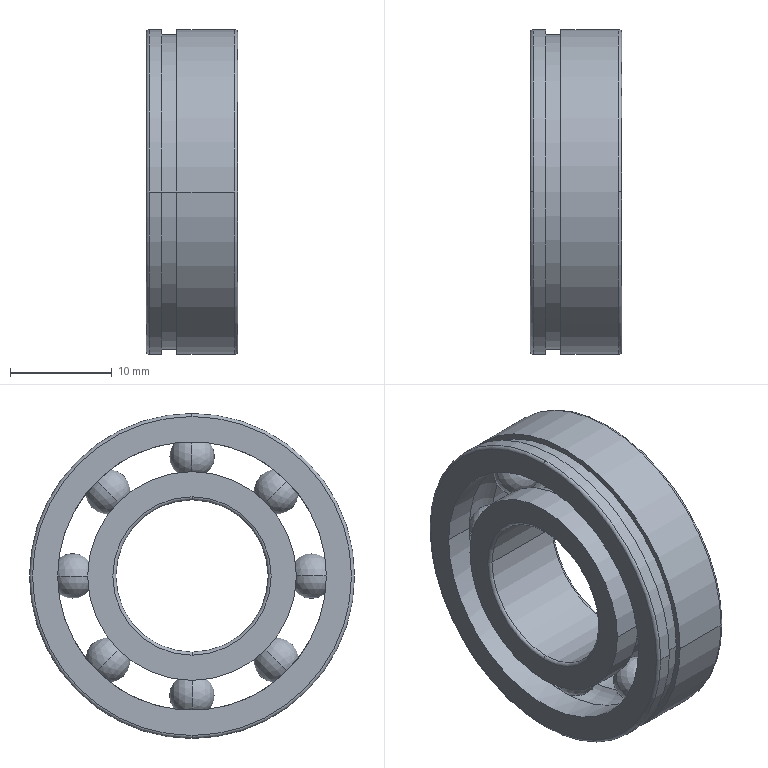Part | SolidWorks | features BaseBody 10 | 10 solids | 52 faces | box 9 x 32 x 32 mm | volume 3713 mm3 | sphere 16 | cylinder 16 | torus 14 | plane 6 | commonest cylinder face diameters 20.542 x4 26.458 x4 32 x4 15 x2 30.92 x2
STEP:
#1=CARTESIAN_POINT('',(4.5,9.54,0.));
#2=VERTEX_POINT('',#1);
#3=CARTESIAN_POINT('',(4.5,13.96,0.));
#4=VERTEX_POINT('',#3);
#5=CARTESIAN_POINT('',(4.5,11.75,0.));
#6=DIRECTION('',(0.,0.,1.));
#7=DIRECTION('',(1.,0.,0.));
#8=AXIS2_PLACEMENT_3D('',#5,#6,#7);
#9=CIRCLE('',#8,2.21);
#10=EDGE_CURVE('',#2,#4,#9,.T.);
#11=ORIENTED_EDGE('',*,*,#10,.F.);
#12=CARTESIAN_POINT('',(4.5,11.75,0.));
#13=DIRECTION('',(0.,0.,-1.));
#14=DIRECTION('',(-1.,0.,0.));
#15=AXIS2_PLACEMENT_3D('',#12,#13,#14);
#16=CIRCLE('',#15,2.21);
#17=EDGE_CURVE('',#2,#4,#16,.T.);
#18=ORIENTED_EDGE('',*,*,#17,.T.);
#19=EDGE_LOOP('',(#11,#18));
#20=FACE_OUTER_BOUND('',#19,.T.);
#21=CARTESIAN_POINT('',(4.5,11.75,0.));
#22=DIRECTION('',(0.,0.,-1.));
#23=DIRECTION('',(1.,0.,0.));
#24=AXIS2_PLACEMENT_3D('',#21,#22,#23);
#25=SPHERICAL_SURFACE('',#24,2.21);
#26=ADVANCED_FACE('',(#20),#25,.T.);
#27=ORIENTED_EDGE('',*,*,#17,.F.);
#28=ORIENTED_EDGE('',*,*,#10,.T.);
#29=EDGE_LOOP('',(#27,#28));
#30=FACE_OUTER_BOUND('',#29,.T.);
#31=CARTESIAN_POINT('',(4.5,11.75,0.));
#32=DIRECTION('',(0.,0.,-1.));
#33=DIRECTION('',(1.,0.,0.));
#34=AXIS2_PLACEMENT_3D('',#31,#32,#33);
#35=SPHERICAL_SURFACE('',#34,2.21);
#36=ADVANCED_FACE('',(#30),#35,.T.);
#37=CLOSED_SHELL('',(#26,#36));
#38=MANIFOLD_SOLID_BREP('',#37);
#39=CARTESIAN_POINT('',(3.,-15.46,0.));
#40=VERTEX_POINT('',#39);
#41=CARTESIAN_POINT('',(3.,15.46,0.));
#42=VERTEX_POINT('',#41);
#43=CARTESIAN_POINT('',(3.,0.,0.));
#44=DIRECTION('',(1.,0.,0.));
#45=DIRECTION('',(0.,1.,0.));
#46=AXIS2_PLACEMENT_3D('',#43,#44,#45);
#47=CIRCLE('',#46,15.46);
#48=EDGE_CURVE('',#40,#42,#47,.T.);
#49=ORIENTED_EDGE('',*,*,#48,.F.);
#50=CARTESIAN_POINT('',(1.5,-15.46,0.));
#51=VERTEX_POINT('',#50);
#52=CARTESIAN_POINT('',(2.25,-15.46,0.));
#53=DIRECTION('',(-1.,0.,0.));
#54=VECTOR('',#53,1000.);
#55=LINE('',#52,#54);
#56=EDGE_CURVE('',#40,#51,#55,.T.);
#57=ORIENTED_EDGE('',*,*,#56,.T.);
#58=CARTESIAN_POINT('',(1.5,15.46,0.));
#59=VERTEX_POINT('',#58);
#60=CARTESIAN_POINT('',(1.5,0.,0.));
#61=DIRECTION('',(1.,0.,0.));
#62=DIRECTION('',(0.,1.,0.));
#63=AXIS2_PLACEMENT_3D('',#60,#61,#62);
#64=CIRCLE('',#63,15.46);
#65=EDGE_CURVE('',#51,#59,#64,.T.);
#66=ORIENTED_EDGE('',*,*,#65,.T.);
#67=CARTESIAN_POINT('',(2.25,15.46,0.));
#68=DIRECTION('',(-1.,0.,0.));
#69=VECTOR('',#68,1000.);
#70=LINE('',#67,#69);
#71=EDGE_CURVE('',#42,#59,#70,.T.);
#72=ORIENTED_EDGE('',*,*,#71,.F.);
#73=EDGE_LOOP('',(#49,#57,#66,#72));
#74=FACE_OUTER_BOUND('',#73,.T.);
#75=CARTESIAN_POINT('',(2.25,0.,0.));
#76=DIRECTION('',(-1.,0.,0.));
#77=DIRECTION('',(0.,1.,0.));
#78=AXIS2_PLACEMENT_3D('',#75,#76,#77);
#79=CYLINDRICAL_SURFACE('',#78,15.46);
#80=ADVANCED_FACE('',(#74),#79,.T.);
#81=CARTESIAN_POINT('',(8.7,-16.,0.));
#82=VERTEX_POINT('',#81);
#83=CARTESIAN_POINT('',(8.7,0.,-16.));
#84=VERTEX_POINT('',#83);
#85=CARTESIAN_POINT('',(8.7,0.,0.));
#86=DIRECTION('',(1.,0.,0.));
#87=DIRECTION('',(0.,-1.,0.));
#88=AXIS2_PLACEMENT_3D('',#85,#86,#87);
#89=CIRCLE('',#88,16.);
#90=EDGE_CURVE('',#82,#84,#89,.T.);
#91=ORIENTED_EDGE('',*,*,#90,.F.);
#92=CARTESIAN_POINT('',(3.,-16.,0.));
#93=VERTEX_POINT('',#92);
#94=CARTESIAN_POINT('',(6.,-16.,0.));
#95=DIRECTION('',(-1.,0.,0.));
#96=VECTOR('',#95,1000.);
#97=LINE('',#94,#96);
#98=EDGE_CURVE('',#82,#93,#97,.T.);
#99=ORIENTED_EDGE('',*,*,#98,.T.);
#100=CARTESIAN_POINT('',(3.,16.,0.));
#101=VERTEX_POINT('',#100);
#102=CARTESIAN_POINT('',(3.,0.,0.));
#103=DIRECTION('',(1.,0.,0.));
#104=DIRECTION('',(0.,1.,0.));
#105=AXIS2_PLACEMENT_3D('',#102,#103,#104);
#106=CIRCLE('',#105,16.);
#107=EDGE_CURVE('',#93,#101,#106,.T.);
#108=ORIENTED_EDGE('',*,*,#107,.T.);
#109=CARTESIAN_POINT('',(8.7,16.,0.));
#110=VERTEX_POINT('',#109);
#111=CARTESIAN_POINT('',(6.,16.,0.));
#112=DIRECTION('',(-1.,0.,0.));
#113=VECTOR('',#112,1000.);
#114=LINE('',#111,#113);
#115=EDGE_CURVE('',#110,#101,#114,.T.);
#116=ORIENTED_EDGE('',*,*,#115,.F.);
#117=CARTESIAN_POINT('',(8.7,0.,0.));
#118=DIRECTION('',(1.,0.,0.));
#119=DIRECTION('',(0.,-1.,0.));
#120=AXIS2_PLACEMENT_3D('',#117,#118,#119);
#121=CIRCLE('',#120,16.);
#122=EDGE_CURVE('',#84,#110,#121,.T.);
#123=ORIENTED_EDGE('',*,*,#122,.F.);
#124=EDGE_LOOP('',(#91,#99,#108,#116,#123));
#125=FACE_OUTER_BOUND('',#124,.T.);
#126=CARTESIAN_POINT('',(6.,0.,0.));
#127=DIRECTION('',(-1.,0.,0.));
#128=DIRECTION('',(0.,1.,0.));
#129=AXIS2_PLACEMENT_3D('',#126,#127,#128);
#130=CYLINDRICAL_SURFACE('',#129,16.);
#131=ADVANCED_FACE('',(#125),#130,.T.);
#132=CARTESIAN_POINT('',(1.5,-16.,0.));
#133=VERTEX_POINT('',#132);
#134=CARTESIAN_POINT('',(1.5,16.,0.));
#135=VERTEX_POINT('',#134);
#136=CARTESIAN_POINT('',(1.5,0.,0.));
#137=DIRECTION('',(1.,0.,0.));
#138=DIRECTION('',(0.,1.,0.));
#139=AXIS2_PLACEMENT_3D('',#136,#137,#138);
#140=CIRCLE('',#139,16.);
#141=EDGE_CURVE('',#133,#135,#140,.T.);
#142=ORIENTED_EDGE('',*,*,#141,.F.);
#143=CARTESIAN_POINT('',(0.3,-16.,0.));
#144=VERTEX_POINT('',#143);
#145=CARTESIAN_POINT('',(0.75,-16.,0.));
#146=DIRECTION('',(-1.,0.,0.));
#147=VECTOR('',#146,1000.);
#148=LINE('',#145,#147);
#149=EDGE_CURVE('',#133,#144,#148,.T.);
#150=ORIENTED_EDGE('',*,*,#149,.T.);
#151=CARTESIAN_POINT('',(0.3,0.,-16.));
#152=VERTEX_POINT('',#151);
#153=CARTESIAN_POINT('',(0.3,0.,0.));
#154=DIRECTION('',(-1.,0.,0.));
#155=DIRECTION('',(0.,-1.,0.));
#156=AXIS2_PLACEMENT_3D('',#153,#154,#155);
#157=CIRCLE('',#156,16.);
#158=EDGE_CURVE('',#152,#144,#157,.T.);
#159=ORIENTED_EDGE('',*,*,#158,.F.);
#160=CARTESIAN_POINT('',(0.3,16.,0.));
#161=VERTEX_POINT('',#160);
#162=CARTESIAN_POINT('',(0.3,0.,0.));
#163=DIRECTION('',(-1.,0.,0.));
#164=DIRECTION('',(0.,-1.,0.));
#165=AXIS2_PLACEMENT_3D('',#162,#163,#164);
#166=CIRCLE('',#165,16.);
#167=EDGE_CURVE('',#161,#152,#166,.T.);
#168=ORIENTED_EDGE('',*,*,#167,.F.);
#169=CARTESIAN_POINT('',(0.75,16.,0.));
#170=DIRECTION('',(-1.,0.,0.));
#171=VECTOR('',#170,1000.);
#172=LINE('',#169,#171);
#173=EDGE_CURVE('',#135,#161,#172,.T.);
#174=ORIENTED_EDGE('',*,*,#173,.F.);
#175=EDGE_LOOP('',(#142,#150,#159,#168,#174));
#176=FACE_OUTER_BOUND('',#175,.T.);
#177=CARTESIAN_POINT('',(0.75,0.,0.));
#178=DIRECTION('',(-1.,0.,0.));
#179=DIRECTION('',(0.,1.,0.));
#180=AXIS2_PLACEMENT_3D('',#177,#178,#179);
#181=CYLINDRICAL_SURFACE('',#180,16.);
#182=ADVANCED_FACE('',(#176),#181,.T.);
#183=ORIENTED_EDGE('',*,*,#122,.T.);
#184=CARTESIAN_POINT('',(8.7,0.,16.));
#185=VERTEX_POINT('',#184);
#186=CARTESIAN_POINT('',(8.7,0.,0.));
#187=DIRECTION('',(1.,0.,0.));
#188=DIRECTION('',(0.,-1.,0.));
#189=AXIS2_PLACEMENT_3D('',#186,#187,#188);
#190=CIRCLE('',#189,16.);
#191=EDGE_CURVE('',#110,#185,#190,.T.);
#192=ORIENTED_EDGE('',*,*,#191,.T.);
#193=CARTESIAN_POINT('',(9.,0.,15.7));
#194=VERTEX_POINT('',#193);
#195=CARTESIAN_POINT('',(8.7,0.,15.7));
#196=DIRECTION('',(0.,1.,0.));
#197=DIRECTION('',(0.,0.,1.));
#198=AXIS2_PLACEMENT_3D('',#195,#196,#197);
#199=CIRCLE('',#198,0.3);
#200=EDGE_CURVE('',#185,#194,#199,.T.);
#201=ORIENTED_EDGE('',*,*,#200,.T.);
#202=CARTESIAN_POINT('',(9.,0.,-15.7));
#203=VERTEX_POINT('',#202);
#204=CARTESIAN_POINT('',(9.,0.,0.));
#205=DIRECTION('',(-1.,0.,0.));
#206=DIRECTION('',(0.,-1.,0.));
#207=AXIS2_PLACEMENT_3D('',#204,#205,#206);
#208=CIRCLE('',#207,15.7);
#209=EDGE_CURVE('',#194,#203,#208,.T.);
#210=ORIENTED_EDGE('',*,*,#209,.T.);
#211=CARTESIAN_POINT('',(8.7,0.,-15.7));
#212=DIRECTION('',(0.,-1.,0.));
#213=DIRECTION('',(0.,0.,-1.));
#214=AXIS2_PLACEMENT_3D('',#211,#212,#213);
#215=CIRCLE('',#214,0.3);
#216=EDGE_CURVE('',#84,#203,#215,.T.);
#217=ORIENTED_EDGE('',*,*,#216,.F.);
#218=EDGE_LOOP('',(#183,#192,#201,#210,#217));
#219=FACE_OUTER_BOUND('',#218,.T.);
#220=CARTESIAN_POINT('',(8.7,0.,0.));
#221=DIRECTION('',(1.,0.,0.));
#222=DIRECTION('',(0.,0.,-1.));
#223=AXIS2_PLACEMENT_3D('',#220,#221,#222);
#224=TOROIDAL_SURFACE('',#223,15.7,0.3);
#225=ADVANCED_FACE('',(#219),#224,.T.);
#226=CARTESIAN_POINT('',(0.,0.,-15.7));
#227=VERTEX_POINT('',#226);
#228=CARTESIAN_POINT('',(0.,0.,15.7));
#229=VERTEX_POINT('',#228);
#230=CARTESIAN_POINT('',(0.,0.,0.));
#231=DIRECTION('',(1.,0.,0.));
#232=DIRECTION('',(0.,-1.,0.));
#233=AXIS2_PLACEMENT_3D('',#230,#231,#232);
#234=CIRCLE('',#233,15.7);
#235=EDGE_CURVE('',#227,#229,#234,.T.);
#236=ORIENTED_EDGE('',*,*,#235,.T.);
#237=CARTESIAN_POINT('',(0.3,0.,16.));
#238=VERTEX_POINT('',#237);
#239=CARTESIAN_POINT('',(0.3,0.,15.7));
#240=DIRECTION('',(0.,1.,0.));
#241=DIRECTION('',(0.,0.,1.));
#242=AXIS2_PLACEMENT_3D('',#239,#240,#241);
#243=CIRCLE('',#242,0.3);
#244=EDGE_CURVE('',#229,#238,#243,.T.);
#245=ORIENTED_EDGE('',*,*,#244,.T.);
#246=CARTESIAN_POINT('',(0.3,0.,0.));
#247=DIRECTION('',(-1.,0.,0.));
#248=DIRECTION('',(0.,-1.,0.));
#249=AXIS2_PLACEMENT_3D('',#246,#247,#248);
#250=CIRCLE('',#249,16.);
#251=EDGE_CURVE('',#238,#161,#250,.T.);
#252=ORIENTED_EDGE('',*,*,#251,.T.);
#253=ORIENTED_EDGE('',*,*,#167,.T.);
#254=CARTESIAN_POINT('',(0.3,0.,-15.7));
#255=DIRECTION('',(0.,-1.,0.));
#256=DIRECTION('',(0.,0.,-1.));
#257=AXIS2_PLACEMENT_3D('',#254,#255,#256);
#258=CIRCLE('',#257,0.3);
#259=EDGE_CURVE('',#227,#152,#258,.T.);
#260=ORIENTED_EDGE('',*,*,#259,.F.);
#261=EDGE_LOOP('',(#236,#245,#252,#253,#260));
#262=FACE_OUTER_BOUND('',#261,.T.);
#263=CARTESIAN_POINT('',(0.3,0.,0.));
#264=DIRECTION('',(1.,0.,0.));
#265=DIRECTION('',(0.,0.,-1.));
#266=AXIS2_PLACEMENT_3D('',#263,#264,#265);
#267=TOROIDAL_SURFACE('',#266,15.7,0.3);
#268=ADVANCED_FACE('',(#262),#267,.T.);
#269=CARTESIAN_POINT('',(9.,13.229,0.));
#270=VERTEX_POINT('',#269);
#271=CARTESIAN_POINT('',(9.,-13.229,0.));
#272=VERTEX_POINT('',#271);
#273=CARTESIAN_POINT('',(9.,0.,0.));
#274=DIRECTION('',(1.,0.,0.));
#275=DIRECTION('',(0.,1.,0.));
#276=AXIS2_PLACEMENT_3D('',#273,#274,#275);
#277=CIRCLE('',#276,13.229);
#278=EDGE_CURVE('',#270,#272,#277,.T.);
#279=ORIENTED_EDGE('',*,*,#278,.T.);
#280=CARTESIAN_POINT('',(6.142,-13.229,0.));
#281=VERTEX_POINT('',#280);
#282=CARTESIAN_POINT('',(7.571,-13.229,0.));
#283=DIRECTION('',(-1.,0.,0.));
#284=VECTOR('',#283,1000.);
#285=LINE('',#282,#284);
#286=EDGE_CURVE('',#272,#281,#285,.T.);
#287=ORIENTED_EDGE('',*,*,#286,.T.);
#288=CARTESIAN_POINT('',(6.142,0.,13.229));
#289=VERTEX_POINT('',#288);
#290=CARTESIAN_POINT('',(6.142,0.,0.));
#291=DIRECTION('',(1.,0.,0.));
#292=DIRECTION('',(0.,1.,0.));
#293=AXIS2_PLACEMENT_3D('',#290,#291,#292);
#294=CIRCLE('',#293,13.229);
#295=EDGE_CURVE('',#289,#281,#294,.T.);
#296=ORIENTED_EDGE('',*,*,#295,.F.);
#297=CARTESIAN_POINT('',(6.142,13.229,0.));
#298=VERTEX_POINT('',#297);
#299=CARTESIAN_POINT('',(6.142,0.,0.));
#300=DIRECTION('',(1.,0.,0.));
#301=DIRECTION('',(0.,1.,0.));
#302=AXIS2_PLACEMENT_3D('',#299,#300,#301);
#303=CIRCLE('',#302,13.229);
#304=EDGE_CURVE('',#298,#289,#303,.T.);
#305=ORIENTED_EDGE('',*,*,#304,.F.);
#306=CARTESIAN_POINT('',(7.571,13.229,0.));
#307=DIRECTION('',(-1.,0.,0.));
#308=VECTOR('',#307,1000.);
#309=LINE('',#306,#308);
#310=EDGE_CURVE('',#270,#298,#309,.T.);
#311=ORIENTED_EDGE('',*,*,#310,.F.);
#312=EDGE_LOOP('',(#279,#287,#296,#305,#311));
#313=FACE_OUTER_BOUND('',#312,.T.);
#314=CARTESIAN_POINT('',(7.571,0.,0.));
#315=DIRECTION('',(-1.,0.,0.));
#316=DIRECTION('',(0.,1.,0.));
#317=AXIS2_PLACEMENT_3D('',#314,#315,#316);
#318=CYLINDRICAL_SURFACE('',#317,13.229);
#319=ADVANCED_FACE('',(#313),#318,.F.);
#320=CARTESIAN_POINT('',(2.858,0.,13.229));
#321=VERTEX_POINT('',#320);
#322=CARTESIAN_POINT('',(2.858,-13.229,0.));
#323=VERTEX_POINT('',#322);
#324=CARTESIAN_POINT('',(2.858,0.,0.));
#325=DIRECTION('',(1.,0.,0.));
#326=DIRECTION('',(0.,1.,0.));
#327=AXIS2_PLACEMENT_3D('',#324,#325,#326);
#328=CIRCLE('',#327,13.229);
#329=EDGE_CURVE('',#321,#323,#328,.T.);
#330=ORIENTED_EDGE('',*,*,#329,.T.);
#331=CARTESIAN_POINT('',(0.,-13.229,0.));
#332=VERTEX_POINT('',#331);
#333=CARTESIAN_POINT('',(1.429,-13.229,0.));
#334=DIRECTION('',(-1.,0.,0.));
#335=VECTOR('',#334,1000.);
#336=LINE('',#333,#335);
#337=EDGE_CURVE('',#323,#332,#336,.T.);
#338=ORIENTED_EDGE('',*,*,#337,.T.);
#339=CARTESIAN_POINT('',(0.,13.229,0.));
#340=VERTEX_POINT('',#339);
#341=CARTESIAN_POINT('',(0.,0.,0.));
#342=DIRECTION('',(1.,0.,0.));
#343=DIRECTION('',(0.,1.,0.));
#344=AXIS2_PLACEMENT_3D('',#341,#342,#343);
#345=CIRCLE('',#344,13.229);
#346=EDGE_CURVE('',#340,#332,#345,.T.);
#347=ORIENTED_EDGE('',*,*,#346,.F.);
#348=CARTESIAN_POINT('',(2.858,13.229,0.));
#349=VERTEX_POINT('',#348);
#350=CARTESIAN_POINT('',(1.429,13.229,0.));
#351=DIRECTION('',(-1.,0.,0.));
#352=VECTOR('',#351,1000.);
#353=LINE('',#350,#352);
#354=EDGE_CURVE('',#349,#340,#353,.T.);
#355=ORIENTED_EDGE('',*,*,#354,.F.);
#356=CARTESIAN_POINT('',(2.858,0.,0.));
#357=DIRECTION('',(1.,0.,0.));
#358=DIRECTION('',(0.,1.,0.));
#359=AXIS2_PLACEMENT_3D('',#356,#357,#358);
#360=CIRCLE('',#359,13.229);
#361=EDGE_CURVE('',#349,#321,#360,.T.);
#362=ORIENTED_EDGE('',*,*,#361,.T.);
#363=EDGE_LOOP('',(#330,#338,#347,#355,#362));
#364=FACE_OUTER_BOUND('',#363,.T.);
#365=CARTESIAN_POINT('',(1.429,0.,0.));
#366=DIRECTION('',(-1.,0.,0.));
#367=DIRECTION('',(0.,1.,0.));
#368=AXIS2_PLACEMENT_3D('',#365,#366,#367);
#369=CYLINDRICAL_SURFACE('',#368,13.229);
#370=ADVANCED_FACE('',(#364),#369,.F.);
#371=ORIENTED_EDGE('',*,*,#329,.F.);
#372=CARTESIAN_POINT('',(4.5,0.,11.75));
#373=DIRECTION('',(0.,1.,0.));
#374=DIRECTION('',(0.,0.,1.));
#375=AXIS2_PLACEMENT_3D('',#372,#373,#374);
#376=CIRCLE('',#375,2.21);
#377=EDGE_CURVE('',#321,#289,#376,.T.);
#378=ORIENTED_EDGE('',*,*,#377,.T.);
#379=ORIENTED_EDGE('',*,*,#295,.T.);
#380=CARTESIAN_POINT('',(6.142,0.,-13.229));
#381=VERTEX_POINT('',#380);
#382=CARTESIAN_POINT('',(6.142,0.,0.));
#383=DIRECTION('',(1.,0.,0.));
#384=DIRECTION('',(0.,1.,0.));
#385=AXIS2_PLACEMENT_3D('',#382,#383,#384);
#386=CIRCLE('',#385,13.229);
#387=EDGE_CURVE('',#281,#381,#386,.T.);
#388=ORIENTED_EDGE('',*,*,#387,.T.);
#389=CARTESIAN_POINT('',(2.858,0.,-13.229));
#390=VERTEX_POINT('',#389);
#391=CARTESIAN_POINT('',(4.5,0.,-11.75));
#392=DIRECTION('',(0.,-1.,0.));
#393=DIRECTION('',(0.,0.,-1.));
#394=AXIS2_PLACEMENT_3D('',#391,#392,#393);
#395=CIRCLE('',#394,2.21);
#396=EDGE_CURVE('',#390,#381,#395,.T.);
#397=ORIENTED_EDGE('',*,*,#396,.F.);
#398=CARTESIAN_POINT('',(2.858,0.,0.));
#399=DIRECTION('',(1.,0.,0.));
#400=DIRECTION('',(0.,1.,0.));
#401=AXIS2_PLACEMENT_3D('',#398,#399,#400);
#402=CIRCLE('',#401,13.229);
#403=EDGE_CURVE('',#323,#390,#402,.T.);
#404=ORIENTED_EDGE('',*,*,#403,.F.);
#405=EDGE_LOOP('',(#371,#378,#379,#388,#397,#404));
#406=FACE_OUTER_BOUND('',#405,.T.);
#407=CARTESIAN_POINT('',(4.5,0.,0.));
#408=DIRECTION('',(1.,0.,0.));
#409=DIRECTION('',(0.,0.,-1.));
#410=AXIS2_PLACEMENT_3D('',#407,#408,#409);
#411=TOROIDAL_SURFACE('',#410,11.75,2.21);
#412=ADVANCED_FACE('',(#406),#411,.F.);
#413=CARTESIAN_POINT('',(3.,0.,0.));
#414=DIRECTION('',(1.,0.,0.));
#415=DIRECTION('',(0.,1.,0.));
#416=AXIS2_PLACEMENT_3D('',#413,#414,#415);
#417=CIRCLE('',#416,15.46);
#418=EDGE_CURVE('',#42,#40,#417,.T.);
#419=ORIENTED_EDGE('',*,*,#418,.T.);
#420=ORIENTED_EDGE('',*,*,#48,.T.);
#421=EDGE_LOOP('',(#419,#420));
#422=FACE_BOUND('',#421,.T.);
#423=CARTESIAN_POINT('',(3.,0.,0.));
#424=DIRECTION('',(1.,0.,0.));
#425=DIRECTION('',(0.,1.,0.));
#426=AXIS2_PLACEMENT_3D('',#423,#424,#425);
#427=CIRCLE('',#426,16.);
#428=EDGE_CURVE('',#101,#93,#427,.T.);
#429=ORIENTED_EDGE('',*,*,#428,.F.);
#430=ORIENTED_EDGE('',*,*,#107,.F.);
#431=EDGE_LOOP('',(#429,#430));
#432=FACE_OUTER_BOUND('',#431,.T.);
#433=CARTESIAN_POINT('',(3.,15.73,0.));
#434=DIRECTION('',(-1.,0.,0.));
#435=DIRECTION('',(0.,0.,1.));
#436=AXIS2_PLACEMENT_3D('',#433,#434,#435);
#437=PLANE('',#436);
#438=ADVANCED_FACE('',(#422,#432),#437,.T.);
#439=CARTESIAN_POINT('',(1.5,0.,0.));
#440=DIRECTION('',(1.,0.,0.));
#441=DIRECTION('',(0.,1.,0.));
#442=AXIS2_PLACEMENT_3D('',#439,#440,#441);
#443=CIRCLE('',#442,15.46);
#444=EDGE_CURVE('',#59,#51,#443,.T.);
#445=ORIENTED_EDGE('',*,*,#444,.F.);
#446=ORIENTED_EDGE('',*,*,#65,.F.);
#447=EDGE_LOOP('',(#445,#446));
#448=FACE_BOUND('',#447,.T.);
#449=CARTESIAN_POINT('',(1.5,0.,0.));
#450=DIRECTION('',(1.,0.,0.));
#451=DIRECTION('',(0.,1.,0.));
#452=AXIS2_PLACEMENT_3D('',#449,#450,#451);
#453=CIRCLE('',#452,16.);
#454=EDGE_CURVE('',#135,#133,#453,.T.);
#455=ORIENTED_EDGE('',*,*,#454,.T.);
#456=ORIENTED_EDGE('',*,*,#141,.T.);
#457=EDGE_LOOP('',(#455,#456));
#458=FACE_OUTER_BOUND('',#457,.T.);
#459=CARTESIAN_POINT('',(1.5,15.73,0.));
#460=DIRECTION('',(1.,0.,0.));
#461=DIRECTION('',(0.,1.,0.));
#462=AXIS2_PLACEMENT_3D('',#459,#460,#461);
#463=PLANE('',#462);
#464=ADVANCED_FACE('',(#448,#458),#463,.T.);
#465=ORIENTED_EDGE('',*,*,#278,.F.);
#466=CARTESIAN_POINT('',(9.,0.,0.));
#467=DIRECTION('',(1.,0.,0.));
#468=DIRECTION('',(0.,1.,0.));
#469=AXIS2_PLACEMENT_3D('',#466,#467,#468);
#470=CIRCLE('',#469,13.229);
#471=EDGE_CURVE('',#272,#270,#470,.T.);
#472=ORIENTED_EDGE('',*,*,#471,.F.);
#473=EDGE_LOOP('',(#465,#472));
#474=FACE_BOUND('',#473,.T.);
#475=CARTESIAN_POINT('',(9.,0.,0.));
#476=DIRECTION('',(-1.,0.,0.));
#477=DIRECTION('',(0.,-1.,0.));
#478=AXIS2_PLACEMENT_3D('',#475,#476,#477);
#479=CIRCLE('',#478,15.7);
#480=EDGE_CURVE('',#203,#194,#479,.T.);
#481=ORIENTED_EDGE('',*,*,#480,.F.);
#482=ORIENTED_EDGE('',*,*,#209,.F.);
#483=EDGE_LOOP('',(#481,#482));
#484=FACE_OUTER_BOUND('',#483,.T.);
#485=CARTESIAN_POINT('',(9.,14.615,0.));
#486=DIRECTION('',(1.,0.,0.));
#487=DIRECTION('',(0.,1.,0.));
#488=AXIS2_PLACEMENT_3D('',#485,#486,#487);
#489=PLANE('',#488);
#490=ADVANCED_FACE('',(#474,#484),#489,.T.);
#491=ORIENTED_EDGE('',*,*,#346,.T.);
#492=CARTESIAN_POINT('',(0.,0.,0.));
#493=DIRECTION('',(1.,0.,0.));
#494=DIRECTION('',(0.,1.,0.));
#495=AXIS2_PLACEMENT_3D('',#492,#493,#494);
#496=CIRCLE('',#495,13.229);
#497=EDGE_CURVE('',#332,#340,#496,.T.);
#498=ORIENTED_EDGE('',*,*,#497,.T.);
#499=EDGE_LOOP('',(#491,#498));
#500=FACE_BOUND('',#499,.T.);
#501=ORIENTED_EDGE('',*,*,#235,.F.);
#502=CARTESIAN_POINT('',(0.,0.,0.));
#503=DIRECTION('',(1.,0.,0.));
#504=DIRECTION('',(0.,-1.,0.));
#505=AXIS2_PLACEMENT_3D('',#502,#503,#504);
#506=CIRCLE('',#505,15.7);
#507=EDGE_CURVE('',#229,#227,#506,.T.);
#508=ORIENTED_EDGE('',*,*,#507,.F.);
#509=EDGE_LOOP('',(#501,#508));
#510=FACE_OUTER_BOUND('',#509,.T.);
#511=CARTESIAN_POINT('',(0.,14.615,0.));
#512=DIRECTION('',(-1.,0.,0.));
#513=DIRECTION('',(0.,0.,1.));
#514=AXIS2_PLACEMENT_3D('',#511,#512,#513);
#515=PLANE('',#514);
#516=ADVANCED_FACE('',(#500,#510),#515,.T.);
#517=ORIENTED_EDGE('',*,*,#377,.F.);
#518=ORIENTED_EDGE('',*,*,#361,.F.);
#519=CARTESIAN_POINT('',(2.858,0.,0.));
#520=DIRECTION('',(1.,0.,0.));
#521=DIRECTION('',(0.,1.,0.));
#522=AXIS2_PLACEMENT_3D('',#519,#520,#521);
#523=CIRCLE('',#522,13.229);
#524=EDGE_CURVE('',#390,#349,#523,.T.);
#525=ORIENTED_EDGE('',*,*,#524,.F.);
#526=ORIENTED_EDGE('',*,*,#396,.T.);
#527=CARTESIAN_POINT('',(6.142,0.,0.));
#528=DIRECTION('',(1.,0.,0.));
#529=DIRECTION('',(0.,1.,0.));
#530=AXIS2_PLACEMENT_3D('',#527,#528,#529);
#531=CIRCLE('',#530,13.229);
#532=EDGE_CURVE('',#381,#298,#531,.T.);
#533=ORIENTED_EDGE('',*,*,#532,.T.);
#534=ORIENTED_EDGE('',*,*,#304,.T.);
#535=EDGE_LOOP('',(#517,#518,#525,#526,#533,#534));
#536=FACE_OUTER_BOUND('',#535,.T.);
#537=CARTESIAN_POINT('',(4.5,0.,0.));
#538=DIRECTION('',(1.,0.,0.));
#539=DIRECTION('',(0.,0.,-1.));
#540=AXIS2_PLACEMENT_3D('',#537,#538,#539);
#541=TOROIDAL_SURFACE('',#540,11.75,2.21);
#542=ADVANCED_FACE('',(#536),#541,.F.);
#543=ORIENTED_EDGE('',*,*,#337,.F.);
#544=ORIENTED_EDGE('',*,*,#403,.T.);
#545=ORIENTED_EDGE('',*,*,#524,.T.);
#546=ORIENTED_EDGE('',*,*,#354,.T.);
#547=ORIENTED_EDGE('',*,*,#497,.F.);
#548=EDGE_LOOP('',(#543,#544,#545,#546,#547));
#549=FACE_OUTER_BOUND('',#548,.T.);
#550=CARTESIAN_POINT('',(1.429,0.,0.));
#551=DIRECTION('',(-1.,0.,0.));
#552=DIRECTION('',(0.,1.,0.));
#553=AXIS2_PLACEMENT_3D('',#550,#551,#552);
#554=CYLINDRICAL_SURFACE('',#553,13.229);
#555=ADVANCED_FACE('',(#549),#554,.F.);
#556=ORIENTED_EDGE('',*,*,#286,.F.);
#557=ORIENTED_EDGE('',*,*,#471,.T.);
#558=ORIENTED_EDGE('',*,*,#310,.T.);
#559=ORIENTED_EDGE('',*,*,#532,.F.);
#560=ORIENTED_EDGE('',*,*,#387,.F.);
#561=EDGE_LOOP('',(#556,#557,#558,#559,#560));
#562=FACE_OUTER_BOUND('',#561,.T.);
#563=CARTESIAN_POINT('',(7.571,0.,0.));
#564=DIRECTION('',(-1.,0.,0.));
#565=DIRECTION('',(0.,1.,0.));
#566=AXIS2_PLACEMENT_3D('',#563,#564,#565);
#567=CYLINDRICAL_SURFACE('',#566,13.229);
#568=ADVANCED_FACE('',(#562),#567,.F.);
#569=ORIENTED_EDGE('',*,*,#244,.F.);
#570=ORIENTED_EDGE('',*,*,#507,.T.);
#571=ORIENTED_EDGE('',*,*,#259,.T.);
#572=ORIENTED_EDGE('',*,*,#158,.T.);
#573=CARTESIAN_POINT('',(0.3,0.,0.));
#574=DIRECTION('',(-1.,0.,0.));
#575=DIRECTION('',(0.,-1.,0.));
#576=AXIS2_PLACEMENT_3D('',#573,#574,#575);
#577=CIRCLE('',#576,16.);
#578=EDGE_CURVE('',#144,#238,#577,.T.);
#579=ORIENTED_EDGE('',*,*,#578,.T.);
#580=EDGE_LOOP('',(#569,#570,#571,#572,#579));
#581=FACE_OUTER_BOUND('',#580,.T.);
#582=CARTESIAN_POINT('',(0.3,0.,0.));
#583=DIRECTION('',(1.,0.,0.));
#584=DIRECTION('',(0.,0.,-1.));
#585=AXIS2_PLACEMENT_3D('',#582,#583,#584);
#586=TOROIDAL_SURFACE('',#585,15.7,0.3);
#587=ADVANCED_FACE('',(#581),#586,.T.);
#588=ORIENTED_EDGE('',*,*,#200,.F.);
#589=CARTESIAN_POINT('',(8.7,0.,0.));
#590=DIRECTION('',(1.,0.,0.));
#591=DIRECTION('',(0.,-1.,0.));
#592=AXIS2_PLACEMENT_3D('',#589,#590,#591);
#593=CIRCLE('',#592,16.);
#594=EDGE_CURVE('',#185,#82,#593,.T.);
#595=ORIENTED_EDGE('',*,*,#594,.T.);
#596=ORIENTED_EDGE('',*,*,#90,.T.);
#597=ORIENTED_EDGE('',*,*,#216,.T.);
#598=ORIENTED_EDGE('',*,*,#480,.T.);
#599=EDGE_LOOP('',(#588,#595,#596,#597,#598));
#600=FACE_OUTER_BOUND('',#599,.T.);
#601=CARTESIAN_POINT('',(8.7,0.,0.));
#602=DIRECTION('',(1.,0.,0.));
#603=DIRECTION('',(0.,0.,-1.));
#604=AXIS2_PLACEMENT_3D('',#601,#602,#603);
#605=TOROIDAL_SURFACE('',#604,15.7,0.3);
#606=ADVANCED_FACE('',(#600),#605,.T.);
#607=ORIENTED_EDGE('',*,*,#149,.F.);
#608=ORIENTED_EDGE('',*,*,#454,.F.);
#609=ORIENTED_EDGE('',*,*,#173,.T.);
#610=ORIENTED_EDGE('',*,*,#251,.F.);
#611=ORIENTED_EDGE('',*,*,#578,.F.);
#612=EDGE_LOOP('',(#607,#608,#609,#610,#611));
#613=FACE_OUTER_BOUND('',#612,.T.);
#614=CARTESIAN_POINT('',(0.75,0.,0.));
#615=DIRECTION('',(-1.,0.,0.));
#616=DIRECTION('',(0.,1.,0.));
#617=AXIS2_PLACEMENT_3D('',#614,#615,#616);
#618=CYLINDRICAL_SURFACE('',#617,16.);
#619=ADVANCED_FACE('',(#613),#618,.T.);
#620=ORIENTED_EDGE('',*,*,#98,.F.);
#621=ORIENTED_EDGE('',*,*,#594,.F.);
#622=ORIENTED_EDGE('',*,*,#191,.F.);
#623=ORIENTED_EDGE('',*,*,#115,.T.);
#624=ORIENTED_EDGE('',*,*,#428,.T.);
#625=EDGE_LOOP('',(#620,#621,#622,#623,#624));
#626=FACE_OUTER_BOUND('',#625,.T.);
#627=CARTESIAN_POINT('',(6.,0.,0.));
#628=DIRECTION('',(-1.,0.,0.));
#629=DIRECTION('',(0.,1.,0.));
#630=AXIS2_PLACEMENT_3D('',#627,#628,#629);
#631=CYLINDRICAL_SURFACE('',#630,16.);
#632=ADVANCED_FACE('',(#626),#631,.T.);
#633=ORIENTED_EDGE('',*,*,#56,.F.);
#634=ORIENTED_EDGE('',*,*,#418,.F.);
#635=ORIENTED_EDGE('',*,*,#71,.T.);
#636=ORIENTED_EDGE('',*,*,#444,.T.);
#637=EDGE_LOOP('',(#633,#634,#635,#636));
#638=FACE_OUTER_BOUND('',#637,.T.);
#639=CARTESIAN_POINT('',(2.25,0.,0.));
#640=DIRECTION('',(-1.,0.,0.));
#641=DIRECTION('',(0.,1.,0.));
#642=AXIS2_PLACEMENT_3D('',#639,#640,#641);
#643=CYLINDRICAL_SURFACE('',#642,15.46);
#644=ADVANCED_FACE('',(#638),#643,.T.);
#645=CLOSED_SHELL('',(#80,#131,#182,#225,#268,#319,#370,#412,#438,#464,#490,#516,#542,#555,#568,#587,#606,#619,#632,#644));
#646=MANIFOLD_SOLID_BREP('',#645);
#647=CARTESIAN_POINT('',(6.142,0.,-10.271));
#648=VERTEX_POINT('',#647);
#649=CARTESIAN_POINT('',(4.5,0.,-9.54));
#650=VERTEX_POINT('',#649);
#651=CARTESIAN_POINT('',(4.5,0.,-11.75));
#652=DIRECTION('',(0.,-1.,0.));
#653=DIRECTION('',(0.,0.,-1.));
#654=AXIS2_PLACEMENT_3D('',#651,#652,#653);
#655=CIRCLE('',#654,2.21);
#656=EDGE_CURVE('',#648,#650,#655,.T.);
#657=ORIENTED_EDGE('',*,*,#656,.T.);
#658=CARTESIAN_POINT('',(4.5,0.,9.54));
#659=VERTEX_POINT('',#658);
#660=CARTESIAN_POINT('',(4.5,0.,0.));
#661=DIRECTION('',(1.,0.,0.));
#662=DIRECTION('',(0.,0.,-1.));
#663=AXIS2_PLACEMENT_3D('',#660,#661,#662);
#664=CIRCLE('',#663,9.54);
#665=EDGE_CURVE('',#650,#659,#664,.T.);
#666=ORIENTED_EDGE('',*,*,#665,.T.);
#667=CARTESIAN_POINT('',(6.142,0.,10.271));
#668=VERTEX_POINT('',#667);
#669=CARTESIAN_POINT('',(4.5,0.,11.75));
#670=DIRECTION('',(0.,1.,0.));
#671=DIRECTION('',(0.,0.,1.));
#672=AXIS2_PLACEMENT_3D('',#669,#670,#671);
#673=CIRCLE('',#672,2.21);
#674=EDGE_CURVE('',#668,#659,#673,.T.);
#675=ORIENTED_EDGE('',*,*,#674,.F.);
#676=CARTESIAN_POINT('',(6.142,10.271,0.));
#677=VERTEX_POINT('',#676);
#678=CARTESIAN_POINT('',(6.142,0.,0.));
#679=DIRECTION('',(1.,0.,0.));
#680=DIRECTION('',(0.,1.,0.));
#681=AXIS2_PLACEMENT_3D('',#678,#679,#680);
#682=CIRCLE('',#681,10.271);
#683=EDGE_CURVE('',#677,#668,#682,.T.);
#684=ORIENTED_EDGE('',*,*,#683,.F.);
#685=CARTESIAN_POINT('',(6.142,0.,0.));
#686=DIRECTION('',(1.,0.,0.));
#687=DIRECTION('',(0.,1.,0.));
#688=AXIS2_PLACEMENT_3D('',#685,#686,#687);
#689=CIRCLE('',#688,10.271);
#690=EDGE_CURVE('',#648,#677,#689,.T.);
#691=ORIENTED_EDGE('',*,*,#690,.F.);
#692=EDGE_LOOP('',(#657,#666,#675,#684,#691));
#693=FACE_OUTER_BOUND('',#692,.T.);
#694=CARTESIAN_POINT('',(4.5,0.,0.));
#695=DIRECTION('',(1.,0.,0.));
#696=DIRECTION('',(0.,0.,-1.));
#697=AXIS2_PLACEMENT_3D('',#694,#695,#696);
#698=TOROIDAL_SURFACE('',#697,11.75,2.21);
#699=ADVANCED_FACE('',(#693),#698,.F.);
#700=ORIENTED_EDGE('',*,*,#674,.T.);
#701=CARTESIAN_POINT('',(4.5,0.,0.));
#702=DIRECTION('',(1.,0.,0.));
#703=DIRECTION('',(0.,0.,-1.));
#704=AXIS2_PLACEMENT_3D('',#701,#702,#703);
#705=CIRCLE('',#704,9.54);
#706=EDGE_CURVE('',#659,#650,#705,.T.);
#707=ORIENTED_EDGE('',*,*,#706,.T.);
#708=ORIENTED_EDGE('',*,*,#656,.F.);
#709=CARTESIAN_POINT('',(6.142,-10.271,0.));
#710=VERTEX_POINT('',#709);
#711=CARTESIAN_POINT('',(6.142,0.,0.));
#712=DIRECTION('',(1.,0.,0.));
#713=DIRECTION('',(0.,1.,0.));
#714=AXIS2_PLACEMENT_3D('',#711,#712,#713);
#715=CIRCLE('',#714,10.271);
#716=EDGE_CURVE('',#710,#648,#715,.T.);
#717=ORIENTED_EDGE('',*,*,#716,.F.);
#718=CARTESIAN_POINT('',(6.142,0.,0.));
#719=DIRECTION('',(1.,0.,0.));
#720=DIRECTION('',(0.,1.,0.));
#721=AXIS2_PLACEMENT_3D('',#718,#719,#720);
#722=CIRCLE('',#721,10.271);
#723=EDGE_CURVE('',#668,#710,#722,.T.);
#724=ORIENTED_EDGE('',*,*,#723,.F.);
#725=EDGE_LOOP('',(#700,#707,#708,#717,#724));
#726=FACE_OUTER_BOUND('',#725,.T.);
#727=CARTESIAN_POINT('',(4.5,0.,0.));
#728=DIRECTION('',(1.,0.,0.));
#729=DIRECTION('',(0.,0.,-1.));
#730=AXIS2_PLACEMENT_3D('',#727,#728,#729);
#731=TOROIDAL_SURFACE('',#730,11.75,2.21);
#732=ADVANCED_FACE('',(#726),#731,.F.);
#733=ORIENTED_EDGE('',*,*,#706,.F.);
#734=CARTESIAN_POINT('',(2.858,0.,10.271));
#735=VERTEX_POINT('',#734);
#736=CARTESIAN_POINT('',(4.5,0.,11.75));
#737=DIRECTION('',(0.,1.,0.));
#738=DIRECTION('',(0.,0.,1.));
#739=AXIS2_PLACEMENT_3D('',#736,#737,#738);
#740=CIRCLE('',#739,2.21);
#741=EDGE_CURVE('',#659,#735,#740,.T.);
#742=ORIENTED_EDGE('',*,*,#741,.T.);
#743=CARTESIAN_POINT('',(2.858,-10.271,0.));
#744=VERTEX_POINT('',#743);
#745=CARTESIAN_POINT('',(2.858,0.,0.));
#746=DIRECTION('',(1.,0.,0.));
#747=DIRECTION('',(0.,1.,0.));
#748=AXIS2_PLACEMENT_3D('',#745,#746,#747);
#749=CIRCLE('',#748,10.271);
#750=EDGE_CURVE('',#735,#744,#749,.T.);
#751=ORIENTED_EDGE('',*,*,#750,.T.);
#752=CARTESIAN_POINT('',(2.858,0.,-10.271));
#753=VERTEX_POINT('',#752);
#754=CARTESIAN_POINT('',(2.858,0.,0.));
#755=DIRECTION('',(1.,0.,0.));
#756=DIRECTION('',(0.,1.,0.));
#757=AXIS2_PLACEMENT_3D('',#754,#755,#756);
#758=CIRCLE('',#757,10.271);
#759=EDGE_CURVE('',#744,#753,#758,.T.);
#760=ORIENTED_EDGE('',*,*,#759,.T.);
#761=CARTESIAN_POINT('',(4.5,0.,-11.75));
#762=DIRECTION('',(0.,-1.,0.));
#763=DIRECTION('',(0.,0.,-1.));
#764=AXIS2_PLACEMENT_3D('',#761,#762,#763);
#765=CIRCLE('',#764,2.21);
#766=EDGE_CURVE('',#650,#753,#765,.T.);
#767=ORIENTED_EDGE('',*,*,#766,.F.);
#768=EDGE_LOOP('',(#733,#742,#751,#760,#767));
#769=FACE_OUTER_BOUND('',#768,.T.);
#770=CARTESIAN_POINT('',(4.5,0.,0.));
#771=DIRECTION('',(1.,0.,0.));
#772=DIRECTION('',(0.,0.,-1.));
#773=AXIS2_PLACEMENT_3D('',#770,#771,#772);
#774=TOROIDAL_SURFACE('',#773,11.75,2.21);
#775=ADVANCED_FACE('',(#769),#774,.F.);
#776=CARTESIAN_POINT('',(8.7,-7.5,0.));
#777=VERTEX_POINT('',#776);
#778=CARTESIAN_POINT('',(8.7,0.,7.5));
#779=VERTEX_POINT('',#778);
#780=CARTESIAN_POINT('',(8.7,0.,0.));
#781=DIRECTION('',(-1.,0.,0.));
#782=DIRECTION('',(0.,-1.,0.));
#783=AXIS2_PLACEMENT_3D('',#780,#781,#782);
#784=CIRCLE('',#783,7.5);
#785=EDGE_CURVE('',#777,#779,#784,.T.);
#786=ORIENTED_EDGE('',*,*,#785,.F.);
#787=CARTESIAN_POINT('',(0.3,-7.5,0.));
#788=VERTEX_POINT('',#787);
#789=CARTESIAN_POINT('',(4.5,-7.5,0.));
#790=DIRECTION('',(-1.,0.,0.));
#791=VECTOR('',#790,1000.);
#792=LINE('',#789,#791);
#793=EDGE_CURVE('',#777,#788,#792,.T.);
#794=ORIENTED_EDGE('',*,*,#793,.T.);
#795=CARTESIAN_POINT('',(0.3,0.,7.5));
#796=VERTEX_POINT('',#795);
#797=CARTESIAN_POINT('',(0.3,0.,0.));
#798=DIRECTION('',(1.,0.,0.));
#799=DIRECTION('',(0.,-1.,0.));
#800=AXIS2_PLACEMENT_3D('',#797,#798,#799);
#801=CIRCLE('',#800,7.5);
#802=EDGE_CURVE('',#796,#788,#801,.T.);
#803=ORIENTED_EDGE('',*,*,#802,.F.);
#804=CARTESIAN_POINT('',(0.3,7.5,0.));
#805=VERTEX_POINT('',#804);
#806=CARTESIAN_POINT('',(0.3,0.,0.));
#807=DIRECTION('',(1.,0.,0.));
#808=DIRECTION('',(0.,-1.,0.));
#809=AXIS2_PLACEMENT_3D('',#806,#807,#808);
#810=CIRCLE('',#809,7.5);
#811=EDGE_CURVE('',#805,#796,#810,.T.);
#812=ORIENTED_EDGE('',*,*,#811,.F.);
#813=CARTESIAN_POINT('',(8.7,7.5,0.));
#814=VERTEX_POINT('',#813);
#815=CARTESIAN_POINT('',(4.5,7.5,0.));
#816=DIRECTION('',(-1.,0.,0.));
#817=VECTOR('',#816,1000.);
#818=LINE('',#815,#817);
#819=EDGE_CURVE('',#814,#805,#818,.T.);
#820=ORIENTED_EDGE('',*,*,#819,.F.);
#821=CARTESIAN_POINT('',(8.7,0.,0.));
#822=DIRECTION('',(-1.,0.,0.));
#823=DIRECTION('',(0.,-1.,0.));
#824=AXIS2_PLACEMENT_3D('',#821,#822,#823);
#825=CIRCLE('',#824,7.5);
#826=EDGE_CURVE('',#779,#814,#825,.T.);
#827=ORIENTED_EDGE('',*,*,#826,.F.);
#828=EDGE_LOOP('',(#786,#794,#803,#812,#820,#827));
#829=FACE_OUTER_BOUND('',#828,.T.);
#830=CARTESIAN_POINT('',(4.5,0.,0.));
#831=DIRECTION('',(-1.,0.,0.));
#832=DIRECTION('',(0.,1.,0.));
#833=AXIS2_PLACEMENT_3D('',#830,#831,#832);
#834=CYLINDRICAL_SURFACE('',#833,7.5);
#835=ADVANCED_FACE('',(#829),#834,.F.);
#836=CARTESIAN_POINT('',(0.3,0.,-7.5));
#837=VERTEX_POINT('',#836);
#838=CARTESIAN_POINT('',(0.3,0.,0.));
#839=DIRECTION('',(1.,0.,0.));
#840=DIRECTION('',(0.,-1.,0.));
#841=AXIS2_PLACEMENT_3D('',#838,#839,#840);
#842=CIRCLE('',#841,7.5);
#843=EDGE_CURVE('',#837,#805,#842,.T.);
#844=ORIENTED_EDGE('',*,*,#843,.T.);
#845=ORIENTED_EDGE('',*,*,#811,.T.);
#846=CARTESIAN_POINT('',(0.,0.,7.8));
#847=VERTEX_POINT('',#846);
#848=CARTESIAN_POINT('',(0.3,0.,7.8));
#849=DIRECTION('',(0.,1.,0.));
#850=DIRECTION('',(0.,0.,1.));
#851=AXIS2_PLACEMENT_3D('',#848,#849,#850);
#852=CIRCLE('',#851,0.3);
#853=EDGE_CURVE('',#796,#847,#852,.T.);
#854=ORIENTED_EDGE('',*,*,#853,.T.);
#855=CARTESIAN_POINT('',(0.,0.,-7.8));
#856=VERTEX_POINT('',#855);
#857=CARTESIAN_POINT('',(0.,0.,0.));
#858=DIRECTION('',(-1.,0.,0.));
#859=DIRECTION('',(0.,-1.,0.));
#860=AXIS2_PLACEMENT_3D('',#857,#858,#859);
#861=CIRCLE('',#860,7.8);
#862=EDGE_CURVE('',#847,#856,#861,.T.);
#863=ORIENTED_EDGE('',*,*,#862,.T.);
#864=CARTESIAN_POINT('',(0.3,0.,-7.8));
#865=DIRECTION('',(0.,-1.,0.));
#866=DIRECTION('',(0.,0.,-1.));
#867=AXIS2_PLACEMENT_3D('',#864,#865,#866);
#868=CIRCLE('',#867,0.3);
#869=EDGE_CURVE('',#837,#856,#868,.T.);
#870=ORIENTED_EDGE('',*,*,#869,.F.);
#871=EDGE_LOOP('',(#844,#845,#854,#863,#870));
#872=FACE_OUTER_BOUND('',#871,.T.);
#873=CARTESIAN_POINT('',(0.3,0.,0.));
#874=DIRECTION('',(1.,0.,0.));
#875=DIRECTION('',(0.,0.,-1.));
#876=AXIS2_PLACEMENT_3D('',#873,#874,#875);
#877=TOROIDAL_SURFACE('',#876,7.8,0.3);
#878=ADVANCED_FACE('',(#872),#877,.T.);
#879=CARTESIAN_POINT('',(9.,0.,-7.8));
#880=VERTEX_POINT('',#879);
#881=CARTESIAN_POINT('',(9.,0.,7.8));
#882=VERTEX_POINT('',#881);
#883=CARTESIAN_POINT('',(9.,0.,0.));
#884=DIRECTION('',(1.,0.,0.));
#885=DIRECTION('',(0.,-1.,0.));
#886=AXIS2_PLACEMENT_3D('',#883,#884,#885);
#887=CIRCLE('',#886,7.8);
#888=EDGE_CURVE('',#880,#882,#887,.T.);
#889=ORIENTED_EDGE('',*,*,#888,.T.);
#890=CARTESIAN_POINT('',(8.7,0.,7.8));
#891=DIRECTION('',(0.,1.,0.));
#892=DIRECTION('',(0.,0.,1.));
#893=AXIS2_PLACEMENT_3D('',#890,#891,#892);
#894=CIRCLE('',#893,0.3);
#895=EDGE_CURVE('',#882,#779,#894,.T.);
#896=ORIENTED_EDGE('',*,*,#895,.T.);
#897=ORIENTED_EDGE('',*,*,#826,.T.);
#898=CARTESIAN_POINT('',(8.7,0.,-7.5));
#899=VERTEX_POINT('',#898);
#900=CARTESIAN_POINT('',(8.7,0.,0.));
#901=DIRECTION('',(-1.,0.,0.));
#902=DIRECTION('',(0.,-1.,0.));
#903=AXIS2_PLACEMENT_3D('',#900,#901,#902);
#904=CIRCLE('',#903,7.5);
#905=EDGE_CURVE('',#814,#899,#904,.T.);
#906=ORIENTED_EDGE('',*,*,#905,.T.);
#907=CARTESIAN_POINT('',(8.7,0.,-7.8));
#908=DIRECTION('',(0.,-1.,0.));
#909=DIRECTION('',(0.,0.,-1.));
#910=AXIS2_PLACEMENT_3D('',#907,#908,#909);
#911=CIRCLE('',#910,0.3);
#912=EDGE_CURVE('',#880,#899,#911,.T.);
#913=ORIENTED_EDGE('',*,*,#912,.F.);
#914=EDGE_LOOP('',(#889,#896,#897,#906,#913));
#915=FACE_OUTER_BOUND('',#914,.T.);
#916=CARTESIAN_POINT('',(8.7,0.,0.));
#917=DIRECTION('',(1.,0.,0.));
#918=DIRECTION('',(0.,0.,-1.));
#919=AXIS2_PLACEMENT_3D('',#916,#917,#918);
#920=TOROIDAL_SURFACE('',#919,7.8,0.3);
#921=ADVANCED_FACE('',(#915),#920,.T.);
#922=ORIENTED_EDGE('',*,*,#759,.F.);
#923=CARTESIAN_POINT('',(0.,-10.271,0.));
#924=VERTEX_POINT('',#923);
#925=CARTESIAN_POINT('',(1.429,-10.271,0.));
#926=DIRECTION('',(-1.,0.,0.));
#927=VECTOR('',#926,1000.);
#928=LINE('',#925,#927);
#929=EDGE_CURVE('',#744,#924,#928,.T.);
#930=ORIENTED_EDGE('',*,*,#929,.T.);
#931=CARTESIAN_POINT('',(0.,10.271,0.));
#932=VERTEX_POINT('',#931);
#933=CARTESIAN_POINT('',(0.,0.,0.));
#934=DIRECTION('',(1.,0.,0.));
#935=DIRECTION('',(0.,1.,0.));
#936=AXIS2_PLACEMENT_3D('',#933,#934,#935);
#937=CIRCLE('',#936,10.271);
#938=EDGE_CURVE('',#924,#932,#937,.T.);
#939=ORIENTED_EDGE('',*,*,#938,.T.);
#940=CARTESIAN_POINT('',(2.858,10.271,0.));
#941=VERTEX_POINT('',#940);
#942=CARTESIAN_POINT('',(1.429,10.271,0.));
#943=DIRECTION('',(-1.,0.,0.));
#944=VECTOR('',#943,1000.);
#945=LINE('',#942,#944);
#946=EDGE_CURVE('',#941,#932,#945,.T.);
#947=ORIENTED_EDGE('',*,*,#946,.F.);
#948=CARTESIAN_POINT('',(2.858,0.,0.));
#949=DIRECTION('',(1.,0.,0.));
#950=DIRECTION('',(0.,1.,0.));
#951=AXIS2_PLACEMENT_3D('',#948,#949,#950);
#952=CIRCLE('',#951,10.271);
#953=EDGE_CURVE('',#753,#941,#952,.T.);
#954=ORIENTED_EDGE('',*,*,#953,.F.);
#955=EDGE_LOOP('',(#922,#930,#939,#947,#954));
#956=FACE_OUTER_BOUND('',#955,.T.);
#957=CARTESIAN_POINT('',(1.429,0.,0.));
#958=DIRECTION('',(-1.,0.,0.));
#959=DIRECTION('',(0.,1.,0.));
#960=AXIS2_PLACEMENT_3D('',#957,#958,#959);
#961=CYLINDRICAL_SURFACE('',#960,10.271);
#962=ADVANCED_FACE('',(#956),#961,.T.);
#963=CARTESIAN_POINT('',(9.,-10.271,0.));
#964=VERTEX_POINT('',#963);
#965=CARTESIAN_POINT('',(9.,10.271,0.));
#966=VERTEX_POINT('',#965);
#967=CARTESIAN_POINT('',(9.,0.,0.));
#968=DIRECTION('',(1.,0.,0.));
#969=DIRECTION('',(0.,1.,0.));
#970=AXIS2_PLACEMENT_3D('',#967,#968,#969);
#971=CIRCLE('',#970,10.271);
#972=EDGE_CURVE('',#964,#966,#971,.T.);
#973=ORIENTED_EDGE('',*,*,#972,.F.);
#974=CARTESIAN_POINT('',(7.571,-10.271,0.));
#975=DIRECTION('',(-1.,0.,0.));
#976=VECTOR('',#975,1000.);
#977=LINE('',#974,#976);
#978=EDGE_CURVE('',#964,#710,#977,.T.);
#979=ORIENTED_EDGE('',*,*,#978,.T.);
#980=ORIENTED_EDGE('',*,*,#716,.T.);
#981=ORIENTED_EDGE('',*,*,#690,.T.);
#982=CARTESIAN_POINT('',(7.571,10.271,0.));
#983=DIRECTION('',(-1.,0.,0.));
#984=VECTOR('',#983,1000.);
#985=LINE('',#982,#984);
#986=EDGE_CURVE('',#966,#677,#985,.T.);
#987=ORIENTED_EDGE('',*,*,#986,.F.);
#988=EDGE_LOOP('',(#973,#979,#980,#981,#987));
#989=FACE_OUTER_BOUND('',#988,.T.);
#990=CARTESIAN_POINT('',(7.571,0.,0.));
#991=DIRECTION('',(-1.,0.,0.));
#992=DIRECTION('',(0.,1.,0.));
#993=AXIS2_PLACEMENT_3D('',#990,#991,#992);
#994=CYLINDRICAL_SURFACE('',#993,10.271);
#995=ADVANCED_FACE('',(#989),#994,.T.);
#996=CARTESIAN_POINT('',(0.,0.,0.));
#997=DIRECTION('',(-1.,0.,0.));
#998=DIRECTION('',(0.,-1.,0.));
#999=AXIS2_PLACEMENT_3D('',#996,#997,#998);
#1000=CIRCLE('',#999,7.8);
#1001=EDGE_CURVE('',#856,#847,#1000,.T.);
#1002=ORIENTED_EDGE('',*,*,#1001,.F.);
#1003=ORIENTED_EDGE('',*,*,#862,.F.);
#1004=EDGE_LOOP('',(#1002,#1003));
#1005=FACE_BOUND('',#1004,.T.);
#1006=CARTESIAN_POINT('',(0.,0.,0.));
#1007=DIRECTION('',(1.,0.,0.));
#1008=DIRECTION('',(0.,1.,0.));
#1009=AXIS2_PLACEMENT_3D('',#1006,#1007,#1008);
#1010=CIRCLE('',#1009,10.271);
#1011=EDGE_CURVE('',#932,#924,#1010,.T.);
#1012=ORIENTED_EDGE('',*,*,#1011,.F.);
#1013=ORIENTED_EDGE('',*,*,#938,.F.);
#1014=EDGE_LOOP('',(#1012,#1013));
#1015=FACE_OUTER_BOUND('',#1014,.T.);
#1016=CARTESIAN_POINT('',(0.,8.885,0.));
#1017=DIRECTION('',(-1.,0.,0.));
#1018=DIRECTION('',(0.,0.,1.));
#1019=AXIS2_PLACEMENT_3D('',#1016,#1017,#1018);
#1020=PLANE('',#1019);
#1021=ADVANCED_FACE('',(#1005,#1015),#1020,.T.);
#1022=ORIENTED_EDGE('',*,*,#888,.F.);
#1023=CARTESIAN_POINT('',(9.,0.,0.));
#1024=DIRECTION('',(1.,0.,0.));
#1025=DIRECTION('',(0.,-1.,0.));
#1026=AXIS2_PLACEMENT_3D('',#1023,#1024,#1025);
#1027=CIRCLE('',#1026,7.8);
#1028=EDGE_CURVE('',#882,#880,#1027,.T.);
#1029=ORIENTED_EDGE('',*,*,#1028,.F.);
#1030=EDGE_LOOP('',(#1022,#1029));
#1031=FACE_BOUND('',#1030,.T.);
#1032=CARTESIAN_POINT('',(9.,0.,0.));
#1033=DIRECTION('',(1.,0.,0.));
#1034=DIRECTION('',(0.,1.,0.));
#1035=AXIS2_PLACEMENT_3D('',#1032,#1033,#1034);
#1036=CIRCLE('',#1035,10.271);
#1037=EDGE_CURVE('',#966,#964,#1036,.T.);
#1038=ORIENTED_EDGE('',*,*,#1037,.T.);
#1039=ORIENTED_EDGE('',*,*,#972,.T.);
#1040=EDGE_LOOP('',(#1038,#1039));
#1041=FACE_OUTER_BOUND('',#1040,.T.);
#1042=CARTESIAN_POINT('',(9.,8.885,0.));
#1043=DIRECTION('',(1.,0.,0.));
#1044=DIRECTION('',(0.,1.,0.));
#1045=AXIS2_PLACEMENT_3D('',#1042,#1043,#1044);
#1046=PLANE('',#1045);
#1047=ADVANCED_FACE('',(#1031,#1041),#1046,.T.);
#1048=ORIENTED_EDGE('',*,*,#978,.F.);
#1049=ORIENTED_EDGE('',*,*,#1037,.F.);
#1050=ORIENTED_EDGE('',*,*,#986,.T.);
#1051=ORIENTED_EDGE('',*,*,#683,.T.);
#1052=ORIENTED_EDGE('',*,*,#723,.T.);
#1053=EDGE_LOOP('',(#1048,#1049,#1050,#1051,#1052));
#1054=FACE_OUTER_BOUND('',#1053,.T.);
#1055=CARTESIAN_POINT('',(7.571,0.,0.));
#1056=DIRECTION('',(-1.,0.,0.));
#1057=DIRECTION('',(0.,1.,0.));
#1058=AXIS2_PLACEMENT_3D('',#1055,#1056,#1057);
#1059=CYLINDRICAL_SURFACE('',#1058,10.271);
#1060=ADVANCED_FACE('',(#1054),#1059,.T.);
#1061=ORIENTED_EDGE('',*,*,#929,.F.);
#1062=ORIENTED_EDGE('',*,*,#750,.F.);
#1063=CARTESIAN_POINT('',(2.858,0.,0.));
#1064=DIRECTION('',(1.,0.,0.));
#1065=DIRECTION('',(0.,1.,0.));
#1066=AXIS2_PLACEMENT_3D('',#1063,#1064,#1065);
#1067=CIRCLE('',#1066,10.271);
#1068=EDGE_CURVE('',#941,#735,#1067,.T.);
#1069=ORIENTED_EDGE('',*,*,#1068,.F.);
#1070=ORIENTED_EDGE('',*,*,#946,.T.);
#1071=ORIENTED_EDGE('',*,*,#1011,.T.);
#1072=EDGE_LOOP('',(#1061,#1062,#1069,#1070,#1071));
#1073=FACE_OUTER_BOUND('',#1072,.T.);
#1074=CARTESIAN_POINT('',(1.429,0.,0.));
#1075=DIRECTION('',(-1.,0.,0.));
#1076=DIRECTION('',(0.,1.,0.));
#1077=AXIS2_PLACEMENT_3D('',#1074,#1075,#1076);
#1078=CYLINDRICAL_SURFACE('',#1077,10.271);
#1079=ADVANCED_FACE('',(#1073),#1078,.T.);
#1080=ORIENTED_EDGE('',*,*,#895,.F.);
#1081=ORIENTED_EDGE('',*,*,#1028,.T.);
#1082=ORIENTED_EDGE('',*,*,#912,.T.);
#1083=CARTESIAN_POINT('',(8.7,0.,0.));
#1084=DIRECTION('',(-1.,0.,0.));
#1085=DIRECTION('',(0.,-1.,0.));
#1086=AXIS2_PLACEMENT_3D('',#1083,#1084,#1085);
#1087=CIRCLE('',#1086,7.5);
#1088=EDGE_CURVE('',#899,#777,#1087,.T.);
#1089=ORIENTED_EDGE('',*,*,#1088,.T.);
#1090=ORIENTED_EDGE('',*,*,#785,.T.);
#1091=EDGE_LOOP('',(#1080,#1081,#1082,#1089,#1090));
#1092=FACE_OUTER_BOUND('',#1091,.T.);
#1093=CARTESIAN_POINT('',(8.7,0.,0.));
#1094=DIRECTION('',(1.,0.,0.));
#1095=DIRECTION('',(0.,0.,-1.));
#1096=AXIS2_PLACEMENT_3D('',#1093,#1094,#1095);
#1097=TOROIDAL_SURFACE('',#1096,7.8,0.3);
#1098=ADVANCED_FACE('',(#1092),#1097,.T.);
#1099=ORIENTED_EDGE('',*,*,#853,.F.);
#1100=ORIENTED_EDGE('',*,*,#802,.T.);
#1101=CARTESIAN_POINT('',(0.3,0.,0.));
#1102=DIRECTION('',(1.,0.,0.));
#1103=DIRECTION('',(0.,-1.,0.));
#1104=AXIS2_PLACEMENT_3D('',#1101,#1102,#1103);
#1105=CIRCLE('',#1104,7.5);
#1106=EDGE_CURVE('',#788,#837,#1105,.T.);
#1107=ORIENTED_EDGE('',*,*,#1106,.T.);
#1108=ORIENTED_EDGE('',*,*,#869,.T.);
#1109=ORIENTED_EDGE('',*,*,#1001,.T.);
#1110=EDGE_LOOP('',(#1099,#1100,#1107,#1108,#1109));
#1111=FACE_OUTER_BOUND('',#1110,.T.);
#1112=CARTESIAN_POINT('',(0.3,0.,0.));
#1113=DIRECTION('',(1.,0.,0.));
#1114=DIRECTION('',(0.,0.,-1.));
#1115=AXIS2_PLACEMENT_3D('',#1112,#1113,#1114);
#1116=TOROIDAL_SURFACE('',#1115,7.8,0.3);
#1117=ADVANCED_FACE('',(#1111),#1116,.T.);
#1118=ORIENTED_EDGE('',*,*,#793,.F.);
#1119=ORIENTED_EDGE('',*,*,#1088,.F.);
#1120=ORIENTED_EDGE('',*,*,#905,.F.);
#1121=ORIENTED_EDGE('',*,*,#819,.T.);
#1122=ORIENTED_EDGE('',*,*,#843,.F.);
#1123=ORIENTED_EDGE('',*,*,#1106,.F.);
#1124=EDGE_LOOP('',(#1118,#1119,#1120,#1121,#1122,#1123));
#1125=FACE_OUTER_BOUND('',#1124,.T.);
#1126=CARTESIAN_POINT('',(4.5,0.,0.));
#1127=DIRECTION('',(-1.,0.,0.));
#1128=DIRECTION('',(0.,1.,0.));
#1129=AXIS2_PLACEMENT_3D('',#1126,#1127,#1128);
#1130=CYLINDRICAL_SURFACE('',#1129,7.5);
#1131=ADVANCED_FACE('',(#1125),#1130,.F.);
#1132=ORIENTED_EDGE('',*,*,#665,.F.);
#1133=ORIENTED_EDGE('',*,*,#766,.T.);
#1134=ORIENTED_EDGE('',*,*,#953,.T.);
#1135=ORIENTED_EDGE('',*,*,#1068,.T.);
#1136=ORIENTED_EDGE('',*,*,#741,.F.);
#1137=EDGE_LOOP('',(#1132,#1133,#1134,#1135,#1136));
#1138=FACE_OUTER_BOUND('',#1137,.T.);
#1139=CARTESIAN_POINT('',(4.5,0.,0.));
#1140=DIRECTION('',(1.,0.,0.));
#1141=DIRECTION('',(0.,0.,-1.));
#1142=AXIS2_PLACEMENT_3D('',#1139,#1140,#1141);
#1143=TOROIDAL_SURFACE('',#1142,11.75,2.21);
#1144=ADVANCED_FACE('',(#1138),#1143,.F.);
#1145=CLOSED_SHELL('',(#699,#732,#775,#835,#878,#921,#962,#995,#1021,#1047,#1060,#1079,#1098,#1117,#1131,#1144));
#1146=MANIFOLD_SOLID_BREP('',#1145);
#1147=CARTESIAN_POINT('',(4.5,6.746,6.746));
#1148=VERTEX_POINT('',#1147);
#1149=CARTESIAN_POINT('',(4.5,9.871,9.871));
#1150=VERTEX_POINT('',#1149);
#1151=CARTESIAN_POINT('',(4.5,8.309,8.309));
#1152=DIRECTION('',(0.,-0.7071,0.7071));
#1153=DIRECTION('',(0.,-0.7071,-0.7071));
#1154=AXIS2_PLACEMENT_3D('',#1151,#1152,#1153);
#1155=CIRCLE('',#1154,2.21);
#1156=EDGE_CURVE('',#1148,#1150,#1155,.T.);
#1157=ORIENTED_EDGE('',*,*,#1156,.F.);
#1158=CARTESIAN_POINT('',(4.5,8.309,8.309));
#1159=DIRECTION('',(0.,0.7071,-0.7071));
#1160=DIRECTION('',(0.,0.7071,0.7071));
#1161=AXIS2_PLACEMENT_3D('',#1158,#1159,#1160);
#1162=CIRCLE('',#1161,2.21);
#1163=EDGE_CURVE('',#1148,#1150,#1162,.T.);
#1164=ORIENTED_EDGE('',*,*,#1163,.T.);
#1165=EDGE_LOOP('',(#1157,#1164));
#1166=FACE_OUTER_BOUND('',#1165,.T.);
#1167=CARTESIAN_POINT('',(4.5,8.309,8.309));
#1168=DIRECTION('',(0.,0.7071,-0.7071));
#1169=DIRECTION('',(1.,0.,0.));
#1170=AXIS2_PLACEMENT_3D('',#1167,#1168,#1169);
#1171=SPHERICAL_SURFACE('',#1170,2.21);
#1172=ADVANCED_FACE('',(#1166),#1171,.T.);
#1173=ORIENTED_EDGE('',*,*,#1163,.F.);
#1174=ORIENTED_EDGE('',*,*,#1156,.T.);
#1175=EDGE_LOOP('',(#1173,#1174));
#1176=FACE_OUTER_BOUND('',#1175,.T.);
#1177=CARTESIAN_POINT('',(4.5,8.309,8.309));
#1178=DIRECTION('',(0.,0.7071,-0.7071));
#1179=DIRECTION('',(1.,0.,0.));
#1180=AXIS2_PLACEMENT_3D('',#1177,#1178,#1179);
#1181=SPHERICAL_SURFACE('',#1180,2.21);
#1182=ADVANCED_FACE('',(#1176),#1181,.T.);
#1183=CLOSED_SHELL('',(#1172,#1182));
#1184=MANIFOLD_SOLID_BREP('',#1183);
#1185=CARTESIAN_POINT('',(4.5,0.,9.54));
#1186=VERTEX_POINT('',#1185);
#1187=CARTESIAN_POINT('',(4.5,0.,13.96));
#1188=VERTEX_POINT('',#1187);
#1189=CARTESIAN_POINT('',(4.5,0.,11.75));
#1190=DIRECTION('',(0.,-1.,0.));
#1191=DIRECTION('',(0.,0.,-1.));
#1192=AXIS2_PLACEMENT_3D('',#1189,#1190,#1191);
#1193=CIRCLE('',#1192,2.21);
#1194=EDGE_CURVE('',#1186,#1188,#1193,.T.);
#1195=ORIENTED_EDGE('',*,*,#1194,.F.);
#1196=CARTESIAN_POINT('',(4.5,0.,11.75));
#1197=DIRECTION('',(0.,1.,0.));
#1198=DIRECTION('',(0.,0.,1.));
#1199=AXIS2_PLACEMENT_3D('',#1196,#1197,#1198);
#1200=CIRCLE('',#1199,2.21);
#1201=EDGE_CURVE('',#1186,#1188,#1200,.T.);
#1202=ORIENTED_EDGE('',*,*,#1201,.T.);
#1203=EDGE_LOOP('',(#1195,#1202));
#1204=FACE_OUTER_BOUND('',#1203,.T.);
#1205=CARTESIAN_POINT('',(4.5,0.,11.75));
#1206=DIRECTION('',(0.,1.,0.));
#1207=DIRECTION('',(1.,0.,0.));
#1208=AXIS2_PLACEMENT_3D('',#1205,#1206,#1207);
#1209=SPHERICAL_SURFACE('',#1208,2.21);
#1210=ADVANCED_FACE('',(#1204),#1209,.T.);
#1211=ORIENTED_EDGE('',*,*,#1201,.F.);
#1212=ORIENTED_EDGE('',*,*,#1194,.T.);
#1213=EDGE_LOOP('',(#1211,#1212));
#1214=FACE_OUTER_BOUND('',#1213,.T.);
#1215=CARTESIAN_POINT('',(4.5,0.,11.75));
#1216=DIRECTION('',(0.,1.,0.));
#1217=DIRECTION('',(1.,0.,0.));
#1218=AXIS2_PLACEMENT_3D('',#1215,#1216,#1217);
#1219=SPHERICAL_SURFACE('',#1218,2.21);
#1220=ADVANCED_FACE('',(#1214),#1219,.T.);
#1221=CLOSED_SHELL('',(#1210,#1220));
#1222=MANIFOLD_SOLID_BREP('',#1221);
#1223=CARTESIAN_POINT('',(4.5,-6.746,6.746));
#1224=VERTEX_POINT('',#1223);
#1225=CARTESIAN_POINT('',(4.5,-9.871,9.871));
#1226=VERTEX_POINT('',#1225);
#1227=CARTESIAN_POINT('',(4.5,-8.309,8.309));
#1228=DIRECTION('',(0.,-0.7071,-0.7071));
#1229=DIRECTION('',(0.,0.7071,-0.7071));
#1230=AXIS2_PLACEMENT_3D('',#1227,#1228,#1229);
#1231=CIRCLE('',#1230,2.21);
#1232=EDGE_CURVE('',#1224,#1226,#1231,.T.);
#1233=ORIENTED_EDGE('',*,*,#1232,.F.);
#1234=CARTESIAN_POINT('',(4.5,-8.309,8.309));
#1235=DIRECTION('',(0.,0.7071,0.7071));
#1236=DIRECTION('',(0.,-0.7071,0.7071));
#1237=AXIS2_PLACEMENT_3D('',#1234,#1235,#1236);
#1238=CIRCLE('',#1237,2.21);
#1239=EDGE_CURVE('',#1224,#1226,#1238,.T.);
#1240=ORIENTED_EDGE('',*,*,#1239,.T.);
#1241=EDGE_LOOP('',(#1233,#1240));
#1242=FACE_OUTER_BOUND('',#1241,.T.);
#1243=CARTESIAN_POINT('',(4.5,-8.309,8.309));
#1244=DIRECTION('',(0.,0.7071,0.7071));
#1245=DIRECTION('',(1.,0.,0.));
#1246=AXIS2_PLACEMENT_3D('',#1243,#1244,#1245);
#1247=SPHERICAL_SURFACE('',#1246,2.21);
#1248=ADVANCED_FACE('',(#1242),#1247,.T.);
#1249=ORIENTED_EDGE('',*,*,#1239,.F.);
#1250=ORIENTED_EDGE('',*,*,#1232,.T.);
#1251=EDGE_LOOP('',(#1249,#1250));
#1252=FACE_OUTER_BOUND('',#1251,.T.);
#1253=CARTESIAN_POINT('',(4.5,-8.309,8.309));
#1254=DIRECTION('',(0.,0.7071,0.7071));
#1255=DIRECTION('',(1.,0.,0.));
#1256=AXIS2_PLACEMENT_3D('',#1253,#1254,#1255);
#1257=SPHERICAL_SURFACE('',#1256,2.21);
#1258=ADVANCED_FACE('',(#1252),#1257,.T.);
#1259=CLOSED_SHELL('',(#1248,#1258));
#1260=MANIFOLD_SOLID_BREP('',#1259);
#1261=CARTESIAN_POINT('',(4.5,-9.54,0.));
#1262=VERTEX_POINT('',#1261);
#1263=CARTESIAN_POINT('',(4.5,-13.96,0.));
#1264=VERTEX_POINT('',#1263);
#1265=CARTESIAN_POINT('',(4.5,-11.75,0.));
#1266=DIRECTION('',(0.,0.,-1.));
#1267=DIRECTION('',(0.,1.,0.));
#1268=AXIS2_PLACEMENT_3D('',#1265,#1266,#1267);
#1269=CIRCLE('',#1268,2.21);
#1270=EDGE_CURVE('',#1262,#1264,#1269,.T.);
#1271=ORIENTED_EDGE('',*,*,#1270,.F.);
#1272=CARTESIAN_POINT('',(4.5,-11.75,0.));
#1273=DIRECTION('',(0.,0.,1.));
#1274=DIRECTION('',(1.,0.,0.));
#1275=AXIS2_PLACEMENT_3D('',#1272,#1273,#1274);
#1276=CIRCLE('',#1275,2.21);
#1277=EDGE_CURVE('',#1262,#1264,#1276,.T.);
#1278=ORIENTED_EDGE('',*,*,#1277,.T.);
#1279=EDGE_LOOP('',(#1271,#1278));
#1280=FACE_OUTER_BOUND('',#1279,.T.);
#1281=CARTESIAN_POINT('',(4.5,-11.75,0.));
#1282=DIRECTION('',(0.,0.,1.));
#1283=DIRECTION('',(1.,0.,0.));
#1284=AXIS2_PLACEMENT_3D('',#1281,#1282,#1283);
#1285=SPHERICAL_SURFACE('',#1284,2.21);
#1286=ADVANCED_FACE('',(#1280),#1285,.T.);
#1287=ORIENTED_EDGE('',*,*,#1277,.F.);
#1288=ORIENTED_EDGE('',*,*,#1270,.T.);
#1289=EDGE_LOOP('',(#1287,#1288));
#1290=FACE_OUTER_BOUND('',#1289,.T.);
#1291=CARTESIAN_POINT('',(4.5,-11.75,0.));
#1292=DIRECTION('',(0.,0.,1.));
#1293=DIRECTION('',(1.,0.,0.));
#1294=AXIS2_PLACEMENT_3D('',#1291,#1292,#1293);
#1295=SPHERICAL_SURFACE('',#1294,2.21);
#1296=ADVANCED_FACE('',(#1290),#1295,.T.);
#1297=CLOSED_SHELL('',(#1286,#1296));
#1298=MANIFOLD_SOLID_BREP('',#1297);
#1299=CARTESIAN_POINT('',(4.5,-6.746,-6.746));
#1300=VERTEX_POINT('',#1299);
#1301=CARTESIAN_POINT('',(4.5,-9.871,-9.871));
#1302=VERTEX_POINT('',#1301);
#1303=CARTESIAN_POINT('',(4.5,-8.309,-8.309));
#1304=DIRECTION('',(0.,0.7071,-0.7071));
#1305=DIRECTION('',(0.,0.7071,0.7071));
#1306=AXIS2_PLACEMENT_3D('',#1303,#1304,#1305);
#1307=CIRCLE('',#1306,2.21);
#1308=EDGE_CURVE('',#1300,#1302,#1307,.T.);
#1309=ORIENTED_EDGE('',*,*,#1308,.F.);
#1310=CARTESIAN_POINT('',(4.5,-8.309,-8.309));
#1311=DIRECTION('',(0.,-0.7071,0.7071));
#1312=DIRECTION('',(0.,-0.7071,-0.7071));
#1313=AXIS2_PLACEMENT_3D('',#1310,#1311,#1312);
#1314=CIRCLE('',#1313,2.21);
#1315=EDGE_CURVE('',#1300,#1302,#1314,.T.);
#1316=ORIENTED_EDGE('',*,*,#1315,.T.);
#1317=EDGE_LOOP('',(#1309,#1316));
#1318=FACE_OUTER_BOUND('',#1317,.T.);
#1319=CARTESIAN_POINT('',(4.5,-8.309,-8.309));
#1320=DIRECTION('',(0.,-0.7071,0.7071));
#1321=DIRECTION('',(1.,0.,0.));
#1322=AXIS2_PLACEMENT_3D('',#1319,#1320,#1321);
#1323=SPHERICAL_SURFACE('',#1322,2.21);
#1324=ADVANCED_FACE('',(#1318),#1323,.T.);
#1325=ORIENTED_EDGE('',*,*,#1315,.F.);
#1326=ORIENTED_EDGE('',*,*,#1308,.T.);
#1327=EDGE_LOOP('',(#1325,#1326));
#1328=FACE_OUTER_BOUND('',#1327,.T.);
#1329=CARTESIAN_POINT('',(4.5,-8.309,-8.309));
#1330=DIRECTION('',(0.,-0.7071,0.7071));
#1331=DIRECTION('',(1.,0.,0.));
#1332=AXIS2_PLACEMENT_3D('',#1329,#1330,#1331);
#1333=SPHERICAL_SURFACE('',#1332,2.21);
#1334=ADVANCED_FACE('',(#1328),#1333,.T.);
#1335=CLOSED_SHELL('',(#1324,#1334));
#1336=MANIFOLD_SOLID_BREP('',#1335);
#1337=CARTESIAN_POINT('',(4.5,0.,-9.54));
#1338=VERTEX_POINT('',#1337);
#1339=CARTESIAN_POINT('',(4.5,0.,-13.96));
#1340=VERTEX_POINT('',#1339);
#1341=CARTESIAN_POINT('',(4.5,0.,-11.75));
#1342=DIRECTION('',(0.,1.,0.));
#1343=DIRECTION('',(0.,0.,1.));
#1344=AXIS2_PLACEMENT_3D('',#1341,#1342,#1343);
#1345=CIRCLE('',#1344,2.21);
#1346=EDGE_CURVE('',#1338,#1340,#1345,.T.);
#1347=ORIENTED_EDGE('',*,*,#1346,.F.);
#1348=CARTESIAN_POINT('',(4.5,0.,-11.75));
#1349=DIRECTION('',(0.,-1.,0.));
#1350=DIRECTION('',(0.,0.,-1.));
#1351=AXIS2_PLACEMENT_3D('',#1348,#1349,#1350);
#1352=CIRCLE('',#1351,2.21);
#1353=EDGE_CURVE('',#1338,#1340,#1352,.T.);
#1354=ORIENTED_EDGE('',*,*,#1353,.T.);
#1355=EDGE_LOOP('',(#1347,#1354));
#1356=FACE_OUTER_BOUND('',#1355,.T.);
#1357=CARTESIAN_POINT('',(4.5,0.,-11.75));
#1358=DIRECTION('',(0.,-1.,0.));
#1359=DIRECTION('',(1.,0.,0.));
#1360=AXIS2_PLACEMENT_3D('',#1357,#1358,#1359);
#1361=SPHERICAL_SURFACE('',#1360,2.21);
#1362=ADVANCED_FACE('',(#1356),#1361,.T.);
#1363=ORIENTED_EDGE('',*,*,#1353,.F.);
#1364=ORIENTED_EDGE('',*,*,#1346,.T.);
#1365=EDGE_LOOP('',(#1363,#1364));
#1366=FACE_OUTER_BOUND('',#1365,.T.);
#1367=CARTESIAN_POINT('',(4.5,0.,-11.75));
#1368=DIRECTION('',(0.,-1.,0.));
#1369=DIRECTION('',(1.,0.,0.));
#1370=AXIS2_PLACEMENT_3D('',#1367,#1368,#1369);
#1371=SPHERICAL_SURFACE('',#1370,2.21);
#1372=ADVANCED_FACE('',(#1366),#1371,.T.);
#1373=CLOSED_SHELL('',(#1362,#1372));
#1374=MANIFOLD_SOLID_BREP('',#1373);
#1375=CARTESIAN_POINT('',(4.5,6.746,-6.746));
#1376=VERTEX_POINT('',#1375);
#1377=CARTESIAN_POINT('',(4.5,9.871,-9.871));
#1378=VERTEX_POINT('',#1377);
#1379=CARTESIAN_POINT('',(4.5,8.309,-8.309));
#1380=DIRECTION('',(0.,0.7071,0.7071));
#1381=DIRECTION('',(0.,-0.7071,0.7071));
#1382=AXIS2_PLACEMENT_3D('',#1379,#1380,#1381);
#1383=CIRCLE('',#1382,2.21);
#1384=EDGE_CURVE('',#1376,#1378,#1383,.T.);
#1385=ORIENTED_EDGE('',*,*,#1384,.F.);
#1386=CARTESIAN_POINT('',(4.5,8.309,-8.309));
#1387=DIRECTION('',(0.,-0.7071,-0.7071));
#1388=DIRECTION('',(0.,0.7071,-0.7071));
#1389=AXIS2_PLACEMENT_3D('',#1386,#1387,#1388);
#1390=CIRCLE('',#1389,2.21);
#1391=EDGE_CURVE('',#1376,#1378,#1390,.T.);
#1392=ORIENTED_EDGE('',*,*,#1391,.T.);
#1393=EDGE_LOOP('',(#1385,#1392));
#1394=FACE_OUTER_BOUND('',#1393,.T.);
#1395=CARTESIAN_POINT('',(4.5,8.309,-8.309));
#1396=DIRECTION('',(0.,-0.7071,-0.7071));
#1397=DIRECTION('',(1.,0.,0.));
#1398=AXIS2_PLACEMENT_3D('',#1395,#1396,#1397);
#1399=SPHERICAL_SURFACE('',#1398,2.21);
#1400=ADVANCED_FACE('',(#1394),#1399,.T.);
#1401=ORIENTED_EDGE('',*,*,#1391,.F.);
#1402=ORIENTED_EDGE('',*,*,#1384,.T.);
#1403=EDGE_LOOP('',(#1401,#1402));
#1404=FACE_OUTER_BOUND('',#1403,.T.);
#1405=CARTESIAN_POINT('',(4.5,8.309,-8.309));
#1406=DIRECTION('',(0.,-0.7071,-0.7071));
#1407=DIRECTION('',(1.,0.,0.));
#1408=AXIS2_PLACEMENT_3D('',#1405,#1406,#1407);
#1409=SPHERICAL_SURFACE('',#1408,2.21);
#1410=ADVANCED_FACE('',(#1404),#1409,.T.);
#1411=CLOSED_SHELL('',(#1400,#1410));
#1412=MANIFOLD_SOLID_BREP('',#1411);
#1413=CARTESIAN_POINT('',(0.,0.,0.));
#1414=DIRECTION('',(0.,0.,1.));
#1415=DIRECTION('',(1.,0.,0.));
#1416=AXIS2_PLACEMENT_3D('',#1413,#1414,#1415);
#1417=(LENGTH_UNIT()NAMED_UNIT(*)SI_UNIT(.MILLI.,.METRE.));
#1418=UNCERTAINTY_MEASURE_WITH_UNIT(LENGTH_MEASURE(0.00001),#1417,'','');
#1419=(NAMED_UNIT(*)PLANE_ANGLE_UNIT()SI_UNIT($,.RADIAN.));
#1420=(NAMED_UNIT(*)SI_UNIT($,.STERADIAN.)SOLID_ANGLE_UNIT());
#1421=(GEOMETRIC_REPRESENTATION_CONTEXT(3)GLOBAL_UNCERTAINTY_ASSIGNED_CONTEXT((#1418))GLOBAL_UNIT_ASSIGNED_CONTEXT((#1417,#1419,#1420))REPRESENTATION_CONTEXT('',''));
#1422=ADVANCED_BREP_SHAPE_REPRESENTATION('',(#38,#646,#1146,#1184,#1222,#1260,#1298,#1336,#1374,#1412,#1416),#1421);